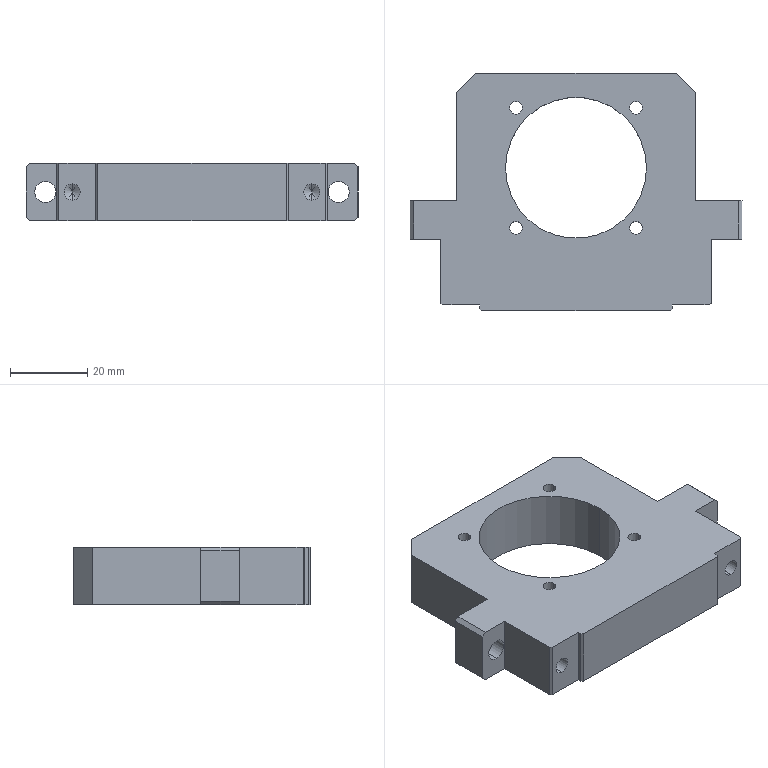Part | SolidWorks | features ICE 7, HoleWzd 4, Chamfer 3, MoveFace 2, Extrusion 1 | 1 solid | 64 faces | box 86 x 61.5 x 15 mm | volume 44493 mm3 | plane 30 | cylinder 26 | cone 8 | commonest cylinder face diameters 3.3 x12 4.2 x4 5.5 x4 9 x4 36.5 x2